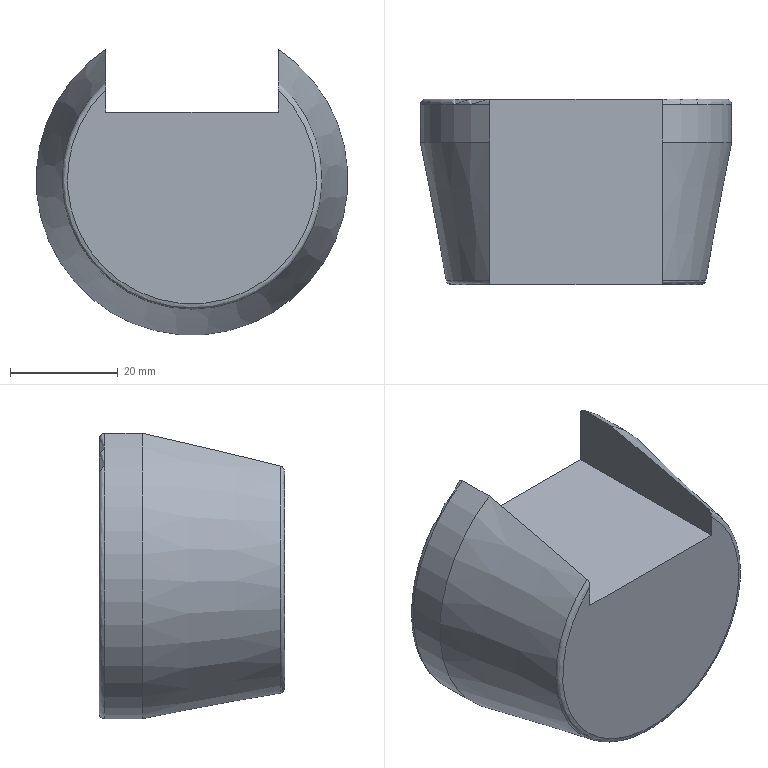Part | NX | features BREP 1 | 1 solid | 12 faces | box 58 x 34.5 x 53.187 mm | volume 61866 mm3 | plane 6 | cylinder 3 | torus 2 | cone 1 | commonest cylinder face diameters 16 x2 58 x1
STEP:
#1=CARTESIAN_POINT('',(16.,-16.5,-33.5));
#2=VERTEX_POINT('',#1);
#3=CARTESIAN_POINT('',(-16.,-16.5,-33.5));
#4=VERTEX_POINT('',#3);
#5=CARTESIAN_POINT('',(16.,-16.5,-33.5));
#6=DIRECTION('',(-1.,0.,0.));
#7=VECTOR('',#6,1000.);
#8=LINE('',#5,#7);
#9=EDGE_CURVE('',#2,#4,#8,.T.);
#10=ORIENTED_EDGE('',*,*,#9,.T.);
#11=CARTESIAN_POINT('',(-16.,-16.5,-29.24));
#12=VERTEX_POINT('',#11);
#13=CARTESIAN_POINT('',(-16.,-16.5,-33.5));
#14=DIRECTION('',(0.,0.,1.));
#15=VECTOR('',#14,1000.);
#16=LINE('',#13,#15);
#17=EDGE_CURVE('',#4,#12,#16,.T.);
#18=ORIENTED_EDGE('',*,*,#17,.T.);
#19=CARTESIAN_POINT('',(16.,-16.5,-29.24));
#20=VERTEX_POINT('',#19);
#21=CARTESIAN_POINT('',(0.,-16.5,-46.));
#22=DIRECTION('',(0.,-1.,0.));
#23=DIRECTION('',(-0.6905,0.,0.7233));
#24=AXIS2_PLACEMENT_3D('',#21,#22,#23);
#25=CIRCLE('',#24,23.171);
#26=EDGE_CURVE('',#12,#20,#25,.T.);
#27=ORIENTED_EDGE('',*,*,#26,.T.);
#28=CARTESIAN_POINT('',(16.,-16.5,-29.24));
#29=DIRECTION('',(0.,0.,-1.));
#30=VECTOR('',#29,1000.);
#31=LINE('',#28,#30);
#32=EDGE_CURVE('',#20,#2,#31,.T.);
#33=ORIENTED_EDGE('',*,*,#32,.T.);
#34=EDGE_LOOP('',(#10,#18,#27,#33));
#35=FACE_BOUND('',#34,.T.);
#36=CARTESIAN_POINT('',(0.,-16.5,-46.));
#37=DIRECTION('',(0.,1.,0.));
#38=DIRECTION('',(1.,0.,0.));
#39=AXIS2_PLACEMENT_3D('',#36,#37,#38);
#40=PLANE('',#39);
#41=ADVANCED_FACE('',(#35),#40,.F.);
#42=CARTESIAN_POINT('',(16.,-15.685,-27.906));
#43=VERTEX_POINT('',#42);
#44=CARTESIAN_POINT('',(16.,-16.5,-29.24));
#45=CARTESIAN_POINT('',(16.,-16.5,-28.539));
#46=CARTESIAN_POINT('',(16.,-16.101,-28.01));
#47=CARTESIAN_POINT('',(16.,-15.685,-27.906));
#48=B_SPLINE_CURVE_WITH_KNOTS('',3,(#44,#45,#46,#47),.UNSPECIFIED.,.F.,.F.,(4,4),(0.,1.),.UNSPECIFIED.);
#49=EDGE_CURVE('',#20,#43,#48,.T.);
#50=ORIENTED_EDGE('',*,*,#49,.T.);
#51=CARTESIAN_POINT('',(16.,10.,-21.813));
#52=VERTEX_POINT('',#51);
#53=CARTESIAN_POINT('',(16.,-15.685,-27.906));
#54=CARTESIAN_POINT('',(16.,-8.357,-26.06));
#55=CARTESIAN_POINT('',(16.,0.2045,-24.029));
#56=CARTESIAN_POINT('',(16.,10.,-21.813));
#57=B_SPLINE_CURVE_WITH_KNOTS('',3,(#53,#54,#55,#56),.UNSPECIFIED.,.F.,.F.,(4,4),(0.,1.),.UNSPECIFIED.);
#58=EDGE_CURVE('',#52,#43,#57,.F.);
#59=ORIENTED_EDGE('',*,*,#58,.F.);
#60=CARTESIAN_POINT('',(16.,17.,-21.813));
#61=VERTEX_POINT('',#60);
#62=CARTESIAN_POINT('',(16.,17.,-21.813));
#63=DIRECTION('',(0.,-1.,0.));
#64=VECTOR('',#63,1000.);
#65=LINE('',#62,#64);
#66=EDGE_CURVE('',#61,#52,#65,.T.);
#67=ORIENTED_EDGE('',*,*,#66,.F.);
#68=CARTESIAN_POINT('',(16.,18.,-23.022));
#69=VERTEX_POINT('',#68);
#70=CARTESIAN_POINT('',(16.,17.,-21.813));
#71=CARTESIAN_POINT('',(16.,17.485,-21.813));
#72=CARTESIAN_POINT('',(16.,18.,-22.313));
#73=CARTESIAN_POINT('',(16.,18.,-23.022));
#74=B_SPLINE_CURVE_WITH_KNOTS('',3,(#70,#71,#72,#73),.UNSPECIFIED.,.F.,.F.,(4,4),(0.,1.),.UNSPECIFIED.);
#75=EDGE_CURVE('',#61,#69,#74,.T.);
#76=ORIENTED_EDGE('',*,*,#75,.T.);
#77=CARTESIAN_POINT('',(16.,18.,-33.5));
#78=VERTEX_POINT('',#77);
#79=CARTESIAN_POINT('',(16.,18.,-23.022));
#80=DIRECTION('',(0.,0.,-1.));
#81=VECTOR('',#80,1000.);
#82=LINE('',#79,#81);
#83=EDGE_CURVE('',#69,#78,#82,.T.);
#84=ORIENTED_EDGE('',*,*,#83,.T.);
#85=CARTESIAN_POINT('',(16.,18.,-33.5));
#86=DIRECTION('',(0.,-1.,0.));
#87=VECTOR('',#86,1000.);
#88=LINE('',#85,#87);
#89=EDGE_CURVE('',#78,#2,#88,.T.);
#90=ORIENTED_EDGE('',*,*,#89,.T.);
#91=ORIENTED_EDGE('',*,*,#32,.F.);
#92=EDGE_LOOP('',(#50,#59,#67,#76,#84,#90,#91));
#93=FACE_BOUND('',#92,.T.);
#94=CARTESIAN_POINT('',(16.,-85.,-33.5));
#95=DIRECTION('',(-1.,0.,0.));
#96=DIRECTION('',(0.,0.,1.));
#97=AXIS2_PLACEMENT_3D('',#94,#95,#96);
#98=PLANE('',#97);
#99=ADVANCED_FACE('',(#93),#98,.T.);
#100=ORIENTED_EDGE('',*,*,#89,.F.);
#101=CARTESIAN_POINT('',(-16.,18.,-33.5));
#102=VERTEX_POINT('',#101);
#103=CARTESIAN_POINT('',(-16.,18.,-33.5));
#104=DIRECTION('',(1.,0.,0.));
#105=VECTOR('',#104,1000.);
#106=LINE('',#103,#105);
#107=EDGE_CURVE('',#102,#78,#106,.T.);
#108=ORIENTED_EDGE('',*,*,#107,.F.);
#109=CARTESIAN_POINT('',(-16.,18.,-33.5));
#110=DIRECTION('',(0.,-1.,0.));
#111=VECTOR('',#110,1000.);
#112=LINE('',#109,#111);
#113=EDGE_CURVE('',#102,#4,#112,.T.);
#114=ORIENTED_EDGE('',*,*,#113,.T.);
#115=ORIENTED_EDGE('',*,*,#9,.F.);
#116=EDGE_LOOP('',(#100,#108,#114,#115));
#117=FACE_BOUND('',#116,.T.);
#118=CARTESIAN_POINT('',(-16.,-85.,-33.5));
#119=DIRECTION('',(0.,0.,1.));
#120=DIRECTION('',(1.,0.,0.));
#121=AXIS2_PLACEMENT_3D('',#118,#119,#120);
#122=PLANE('',#121);
#123=ADVANCED_FACE('',(#117),#122,.T.);
#124=ORIENTED_EDGE('',*,*,#113,.F.);
#125=CARTESIAN_POINT('',(-16.,18.,-23.022));
#126=VERTEX_POINT('',#125);
#127=CARTESIAN_POINT('',(-16.,18.,-23.022));
#128=DIRECTION('',(0.,0.,-1.));
#129=VECTOR('',#128,1000.);
#130=LINE('',#127,#129);
#131=EDGE_CURVE('',#126,#102,#130,.T.);
#132=ORIENTED_EDGE('',*,*,#131,.F.);
#133=CARTESIAN_POINT('',(-16.,17.,-21.813));
#134=VERTEX_POINT('',#133);
#135=CARTESIAN_POINT('',(-16.,18.,-23.022));
#136=CARTESIAN_POINT('',(-16.,18.,-22.675));
#137=CARTESIAN_POINT('',(-16.,17.732,-22.01));
#138=CARTESIAN_POINT('',(-16.,17.234,-21.813));
#139=CARTESIAN_POINT('',(-16.,17.,-21.813));
#140=B_SPLINE_CURVE_WITH_KNOTS('',3,(#135,#136,#137,#138,#139),.UNSPECIFIED.,.F.,.F.,(4,1,4),(0.,0.5,1.),.UNSPECIFIED.);
#141=EDGE_CURVE('',#126,#134,#140,.T.);
#142=ORIENTED_EDGE('',*,*,#141,.T.);
#143=CARTESIAN_POINT('',(-16.,10.,-21.813));
#144=VERTEX_POINT('',#143);
#145=CARTESIAN_POINT('',(-16.,10.,-21.813));
#146=DIRECTION('',(0.,1.,0.));
#147=VECTOR('',#146,1000.);
#148=LINE('',#145,#147);
#149=EDGE_CURVE('',#144,#134,#148,.T.);
#150=ORIENTED_EDGE('',*,*,#149,.F.);
#151=CARTESIAN_POINT('',(-16.,-15.685,-27.906));
#152=VERTEX_POINT('',#151);
#153=CARTESIAN_POINT('',(-16.,10.,-21.813));
#154=CARTESIAN_POINT('',(-16.,0.2045,-24.029));
#155=CARTESIAN_POINT('',(-16.,-8.357,-26.06));
#156=CARTESIAN_POINT('',(-16.,-15.685,-27.906));
#157=B_SPLINE_CURVE_WITH_KNOTS('',3,(#153,#154,#155,#156),.UNSPECIFIED.,.F.,.F.,(4,4),(0.,1.),.UNSPECIFIED.);
#158=EDGE_CURVE('',#152,#144,#157,.F.);
#159=ORIENTED_EDGE('',*,*,#158,.F.);
#160=CARTESIAN_POINT('',(-16.,-15.685,-27.906));
#161=CARTESIAN_POINT('',(-16.,-16.108,-28.012));
#162=CARTESIAN_POINT('',(-16.,-16.5,-28.539));
#163=CARTESIAN_POINT('',(-16.,-16.5,-29.24));
#164=B_SPLINE_CURVE_WITH_KNOTS('',3,(#160,#161,#162,#163),.UNSPECIFIED.,.F.,.F.,(4,4),(0.,1.),.UNSPECIFIED.);
#165=EDGE_CURVE('',#152,#12,#164,.T.);
#166=ORIENTED_EDGE('',*,*,#165,.T.);
#167=ORIENTED_EDGE('',*,*,#17,.F.);
#168=EDGE_LOOP('',(#124,#132,#142,#150,#159,#166,#167));
#169=FACE_BOUND('',#168,.T.);
#170=CARTESIAN_POINT('',(-16.,-85.,-19.448));
#171=DIRECTION('',(1.,0.,0.));
#172=DIRECTION('',(0.,1.,0.));
#173=AXIS2_PLACEMENT_3D('',#170,#171,#172);
#174=PLANE('',#173);
#175=ADVANCED_FACE('',(#169),#174,.T.);
#176=CARTESIAN_POINT('',(0.,-15.685,-46.));
#177=DIRECTION('',(0.,-1.,0.));
#178=DIRECTION('',(-0.6624,0.,-0.7491));
#179=AXIS2_PLACEMENT_3D('',#176,#177,#178);
#180=CIRCLE('',#179,24.154);
#181=EDGE_CURVE('',#152,#43,#180,.T.);
#182=ORIENTED_EDGE('',*,*,#181,.T.);
#183=ORIENTED_EDGE('',*,*,#49,.F.);
#184=ORIENTED_EDGE('',*,*,#26,.F.);
#185=ORIENTED_EDGE('',*,*,#165,.F.);
#186=EDGE_LOOP('',(#182,#183,#184,#185));
#187=FACE_BOUND('',#186,.T.);
#188=CARTESIAN_POINT('',(0.,-15.5,-46.));
#189=DIRECTION('',(0.,1.,0.));
#190=DIRECTION('',(0.6624,0.,0.7491));
#191=AXIS2_PLACEMENT_3D('',#188,#189,#190);
#192=TOROIDAL_SURFACE('',#191,23.171,1.);
#193=ADVANCED_FACE('',(#187),#192,.T.);
#194=ORIENTED_EDGE('',*,*,#58,.T.);
#195=ORIENTED_EDGE('',*,*,#181,.F.);
#196=ORIENTED_EDGE('',*,*,#158,.T.);
#197=CARTESIAN_POINT('',(0.,10.,-46.));
#198=DIRECTION('',(0.,-1.,0.));
#199=DIRECTION('',(-0.5517,0.,0.834));
#200=AXIS2_PLACEMENT_3D('',#197,#198,#199);
#201=CIRCLE('',#200,29.);
#202=EDGE_CURVE('',#144,#52,#201,.T.);
#203=ORIENTED_EDGE('',*,*,#202,.T.);
#204=EDGE_LOOP('',(#194,#195,#196,#203));
#205=FACE_BOUND('',#204,.T.);
#206=CARTESIAN_POINT('',(0.,-2.843,-46.));
#207=DIRECTION('',(0.,1.,0.));
#208=DIRECTION('',(0.5517,0.,0.834));
#209=AXIS2_PLACEMENT_3D('',#206,#207,#208);
#210=CONICAL_SURFACE('',#209,26.577,0.1865);
#211=ADVANCED_FACE('',(#205),#210,.T.);
#212=ORIENTED_EDGE('',*,*,#66,.T.);
#213=ORIENTED_EDGE('',*,*,#202,.F.);
#214=ORIENTED_EDGE('',*,*,#149,.T.);
#215=CARTESIAN_POINT('',(0.,17.,-46.));
#216=DIRECTION('',(0.,1.,0.));
#217=DIRECTION('',(-1.,0.,0.));
#218=AXIS2_PLACEMENT_3D('',#215,#216,#217);
#219=CIRCLE('',#218,29.);
#220=EDGE_CURVE('',#61,#134,#219,.T.);
#221=ORIENTED_EDGE('',*,*,#220,.F.);
#222=EDGE_LOOP('',(#212,#213,#214,#221));
#223=FACE_BOUND('',#222,.T.);
#224=CARTESIAN_POINT('',(0.,103.,-46.));
#225=DIRECTION('',(0.,1.,0.));
#226=DIRECTION('',(0.5517,0.,0.834));
#227=AXIS2_PLACEMENT_3D('',#224,#225,#226);
#228=CYLINDRICAL_SURFACE('',#227,29.);
#229=ADVANCED_FACE('',(#223),#228,.T.);
#230=CARTESIAN_POINT('',(0.,18.,-46.));
#231=DIRECTION('',(0.,1.,0.));
#232=DIRECTION('',(-0.5517,0.,-0.834));
#233=AXIS2_PLACEMENT_3D('',#230,#231,#232);
#234=CIRCLE('',#233,28.);
#235=EDGE_CURVE('',#69,#126,#234,.T.);
#236=ORIENTED_EDGE('',*,*,#235,.F.);
#237=ORIENTED_EDGE('',*,*,#75,.F.);
#238=ORIENTED_EDGE('',*,*,#220,.T.);
#239=ORIENTED_EDGE('',*,*,#141,.F.);
#240=EDGE_LOOP('',(#236,#237,#238,#239));
#241=FACE_BOUND('',#240,.T.);
#242=CARTESIAN_POINT('',(0.,17.,-46.));
#243=DIRECTION('',(0.,1.,0.));
#244=DIRECTION('',(0.5517,0.,0.834));
#245=AXIS2_PLACEMENT_3D('',#242,#243,#244);
#246=TOROIDAL_SURFACE('',#245,28.,1.);
#247=ADVANCED_FACE('',(#241),#246,.T.);
#248=ORIENTED_EDGE('',*,*,#83,.F.);
#249=ORIENTED_EDGE('',*,*,#235,.T.);
#250=ORIENTED_EDGE('',*,*,#131,.T.);
#251=ORIENTED_EDGE('',*,*,#107,.T.);
#252=EDGE_LOOP('',(#248,#249,#250,#251));
#253=FACE_BOUND('',#252,.T.);
#254=CARTESIAN_POINT('',(0.,18.,-54.));
#255=VERTEX_POINT('',#254);
#256=CARTESIAN_POINT('',(0.,18.,-38.));
#257=VERTEX_POINT('',#256);
#258=CARTESIAN_POINT('',(0.,18.,-46.));
#259=DIRECTION('',(0.,-1.,0.));
#260=DIRECTION('',(0.,0.,-1.));
#261=AXIS2_PLACEMENT_3D('',#258,#259,#260);
#262=CIRCLE('',#261,8.);
#263=EDGE_CURVE('',#255,#257,#262,.T.);
#264=ORIENTED_EDGE('',*,*,#263,.T.);
#265=CARTESIAN_POINT('',(0.,18.,-46.));
#266=DIRECTION('',(0.,-1.,0.));
#267=DIRECTION('',(0.,0.,1.));
#268=AXIS2_PLACEMENT_3D('',#265,#266,#267);
#269=CIRCLE('',#268,8.);
#270=EDGE_CURVE('',#257,#255,#269,.T.);
#271=ORIENTED_EDGE('',*,*,#270,.T.);
#272=EDGE_LOOP('',(#264,#271));
#273=FACE_BOUND('',#272,.T.);
#274=CARTESIAN_POINT('',(0.,18.,-18.));
#275=DIRECTION('',(0.,-1.,0.));
#276=DIRECTION('',(0.,0.,-1.));
#277=AXIS2_PLACEMENT_3D('',#274,#275,#276);
#278=PLANE('',#277);
#279=ADVANCED_FACE('',(#253,#273),#278,.F.);
#280=ORIENTED_EDGE('',*,*,#270,.F.);
#281=CARTESIAN_POINT('',(0.,0.,-38.));
#282=VERTEX_POINT('',#281);
#283=CARTESIAN_POINT('',(0.,18.,-38.));
#284=DIRECTION('',(0.,-1.,0.));
#285=VECTOR('',#284,1000.);
#286=LINE('',#283,#285);
#287=EDGE_CURVE('',#257,#282,#286,.T.);
#288=ORIENTED_EDGE('',*,*,#287,.T.);
#289=CARTESIAN_POINT('',(0.,0.,-54.));
#290=VERTEX_POINT('',#289);
#291=CARTESIAN_POINT('',(0.,0.,-46.));
#292=DIRECTION('',(0.,1.,0.));
#293=DIRECTION('',(0.,0.,-1.));
#294=AXIS2_PLACEMENT_3D('',#291,#292,#293);
#295=CIRCLE('',#294,8.);
#296=EDGE_CURVE('',#290,#282,#295,.T.);
#297=ORIENTED_EDGE('',*,*,#296,.F.);
#298=CARTESIAN_POINT('',(0.,18.,-54.));
#299=DIRECTION('',(0.,-1.,0.));
#300=VECTOR('',#299,1000.);
#301=LINE('',#298,#300);
#302=EDGE_CURVE('',#255,#290,#301,.T.);
#303=ORIENTED_EDGE('',*,*,#302,.F.);
#304=EDGE_LOOP('',(#280,#288,#297,#303));
#305=FACE_BOUND('',#304,.T.);
#306=CARTESIAN_POINT('',(0.,103.,-46.));
#307=DIRECTION('',(0.,1.,0.));
#308=DIRECTION('',(0.,0.,-1.));
#309=AXIS2_PLACEMENT_3D('',#306,#307,#308);
#310=CYLINDRICAL_SURFACE('',#309,8.);
#311=ADVANCED_FACE('',(#305),#310,.F.);
#312=CARTESIAN_POINT('',(0.,0.,-46.));
#313=DIRECTION('',(0.,1.,0.));
#314=DIRECTION('',(0.,0.,1.));
#315=AXIS2_PLACEMENT_3D('',#312,#313,#314);
#316=CIRCLE('',#315,8.);
#317=EDGE_CURVE('',#282,#290,#316,.T.);
#318=ORIENTED_EDGE('',*,*,#317,.F.);
#319=ORIENTED_EDGE('',*,*,#287,.F.);
#320=ORIENTED_EDGE('',*,*,#263,.F.);
#321=ORIENTED_EDGE('',*,*,#302,.T.);
#322=EDGE_LOOP('',(#318,#319,#320,#321));
#323=FACE_BOUND('',#322,.T.);
#324=CARTESIAN_POINT('',(0.,103.,-46.));
#325=DIRECTION('',(0.,1.,0.));
#326=DIRECTION('',(0.,0.,1.));
#327=AXIS2_PLACEMENT_3D('',#324,#325,#326);
#328=CYLINDRICAL_SURFACE('',#327,8.);
#329=ADVANCED_FACE('',(#323),#328,.F.);
#330=ORIENTED_EDGE('',*,*,#296,.T.);
#331=ORIENTED_EDGE('',*,*,#317,.T.);
#332=EDGE_LOOP('',(#330,#331));
#333=FACE_BOUND('',#332,.T.);
#334=CARTESIAN_POINT('',(0.,0.,-46.));
#335=DIRECTION('',(0.,1.,0.));
#336=DIRECTION('',(1.,0.,0.));
#337=AXIS2_PLACEMENT_3D('',#334,#335,#336);
#338=PLANE('',#337);
#339=ADVANCED_FACE('',(#333),#338,.T.);
#340=CLOSED_SHELL('',(#41,#99,#123,#175,#193,#211,#229,#247,#279,#311,#329,#339));
#341=MANIFOLD_SOLID_BREP('',#340);
#342=(LENGTH_UNIT()NAMED_UNIT(*)SI_UNIT(.MILLI.,.METRE.));
#343=UNCERTAINTY_MEASURE_WITH_UNIT(LENGTH_MEASURE(0.0508),#342,'','');
#344=(NAMED_UNIT(*)PLANE_ANGLE_UNIT()SI_UNIT($,.RADIAN.));
#345=(NAMED_UNIT(*)SI_UNIT($,.STERADIAN.)SOLID_ANGLE_UNIT());
#346=(GEOMETRIC_REPRESENTATION_CONTEXT(3)GLOBAL_UNCERTAINTY_ASSIGNED_CONTEXT((#343))GLOBAL_UNIT_ASSIGNED_CONTEXT((#342,#344,#345))REPRESENTATION_CONTEXT('',''));
#347=ADVANCED_BREP_SHAPE_REPRESENTATION('',(#341),#346);